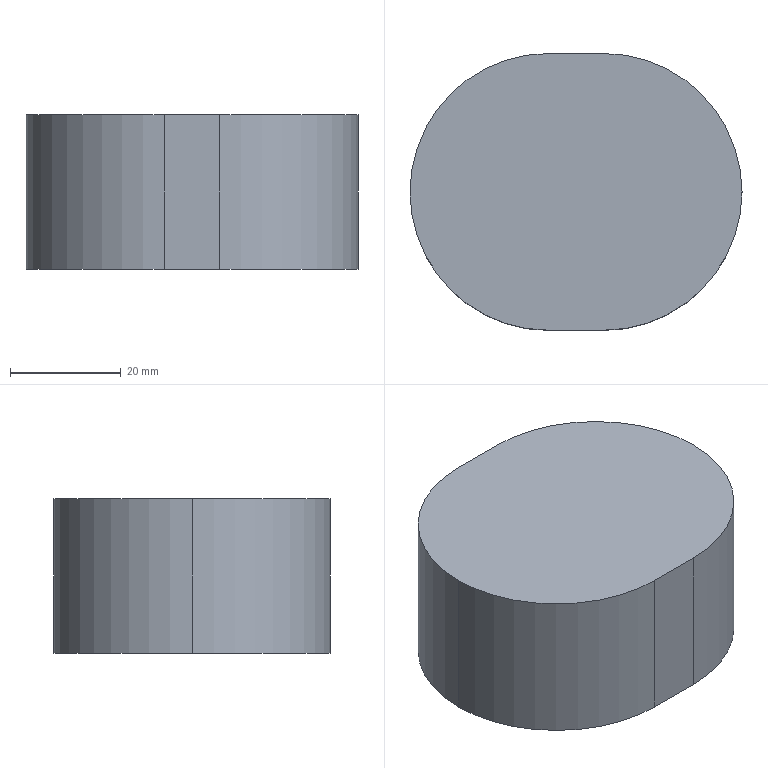Part | SolidWorks | features Extrusion 1, Fillet 1 | 1 solid | 8 faces | box 60 x 50 x 28 mm | volume 68978 mm3 | plane 4 | cylinder 4 | commonest cylinder face diameters 50 x4
STEP:
#1=CARTESIAN_POINT('',(5.,25.,28.));
#2=VERTEX_POINT('',#1);
#3=CARTESIAN_POINT('',(-5.,25.,28.));
#4=VERTEX_POINT('',#3);
#5=CARTESIAN_POINT('',(-30.,25.,28.));
#6=DIRECTION('',(-1.,0.,0.));
#7=VECTOR('',#6,1000.);
#8=LINE('',#5,#7);
#9=EDGE_CURVE('',#2,#4,#8,.T.);
#10=ORIENTED_EDGE('',*,*,#9,.F.);
#11=CARTESIAN_POINT('',(5.,25.,0.));
#12=VERTEX_POINT('',#11);
#13=CARTESIAN_POINT('',(5.,25.,28.));
#14=DIRECTION('',(0.,0.,-1.));
#15=VECTOR('',#14,1000.);
#16=LINE('',#13,#15);
#17=EDGE_CURVE('',#2,#12,#16,.T.);
#18=ORIENTED_EDGE('',*,*,#17,.T.);
#19=CARTESIAN_POINT('',(-5.,25.,0.));
#20=VERTEX_POINT('',#19);
#21=CARTESIAN_POINT('',(-30.,25.,0.));
#22=DIRECTION('',(-1.,0.,0.));
#23=VECTOR('',#22,1000.);
#24=LINE('',#21,#23);
#25=EDGE_CURVE('',#12,#20,#24,.T.);
#26=ORIENTED_EDGE('',*,*,#25,.T.);
#27=CARTESIAN_POINT('',(-5.,25.,28.));
#28=DIRECTION('',(0.,0.,1.));
#29=VECTOR('',#28,1000.);
#30=LINE('',#27,#29);
#31=EDGE_CURVE('',#20,#4,#30,.T.);
#32=ORIENTED_EDGE('',*,*,#31,.T.);
#33=EDGE_LOOP('',(#10,#18,#26,#32));
#34=FACE_OUTER_BOUND('',#33,.T.);
#35=CARTESIAN_POINT('',(-30.,25.,28.));
#36=DIRECTION('',(0.,-1.,0.));
#37=DIRECTION('',(0.,0.,-1.));
#38=AXIS2_PLACEMENT_3D('',#35,#36,#37);
#39=PLANE('',#38);
#40=ADVANCED_FACE('',(#34),#39,.F.);
#41=CARTESIAN_POINT('',(-5.,-25.,0.));
#42=VERTEX_POINT('',#41);
#43=CARTESIAN_POINT('',(5.,-25.,0.));
#44=VERTEX_POINT('',#43);
#45=CARTESIAN_POINT('',(-30.,-25.,0.));
#46=DIRECTION('',(1.,0.,0.));
#47=VECTOR('',#46,1000.);
#48=LINE('',#45,#47);
#49=EDGE_CURVE('',#42,#44,#48,.T.);
#50=ORIENTED_EDGE('',*,*,#49,.T.);
#51=CARTESIAN_POINT('',(5.,-25.,28.));
#52=VERTEX_POINT('',#51);
#53=CARTESIAN_POINT('',(5.,-25.,28.));
#54=DIRECTION('',(0.,0.,1.));
#55=VECTOR('',#54,1000.);
#56=LINE('',#53,#55);
#57=EDGE_CURVE('',#44,#52,#56,.T.);
#58=ORIENTED_EDGE('',*,*,#57,.T.);
#59=CARTESIAN_POINT('',(-5.,-25.,28.));
#60=VERTEX_POINT('',#59);
#61=CARTESIAN_POINT('',(-30.,-25.,28.));
#62=DIRECTION('',(1.,0.,0.));
#63=VECTOR('',#62,1000.);
#64=LINE('',#61,#63);
#65=EDGE_CURVE('',#60,#52,#64,.T.);
#66=ORIENTED_EDGE('',*,*,#65,.F.);
#67=CARTESIAN_POINT('',(-5.,-25.,28.));
#68=DIRECTION('',(0.,0.,-1.));
#69=VECTOR('',#68,1000.);
#70=LINE('',#67,#69);
#71=EDGE_CURVE('',#60,#42,#70,.T.);
#72=ORIENTED_EDGE('',*,*,#71,.T.);
#73=EDGE_LOOP('',(#50,#58,#66,#72));
#74=FACE_OUTER_BOUND('',#73,.T.);
#75=CARTESIAN_POINT('',(-30.,-25.,28.));
#76=DIRECTION('',(0.,1.,0.));
#77=DIRECTION('',(0.,0.,1.));
#78=AXIS2_PLACEMENT_3D('',#75,#76,#77);
#79=PLANE('',#78);
#80=ADVANCED_FACE('',(#74),#79,.F.);
#81=ORIENTED_EDGE('',*,*,#65,.T.);
#82=CARTESIAN_POINT('',(30.,0.,28.));
#83=VERTEX_POINT('',#82);
#84=CARTESIAN_POINT('',(5.,0.,28.));
#85=DIRECTION('',(0.,0.,1.));
#86=DIRECTION('',(1.,0.,0.));
#87=AXIS2_PLACEMENT_3D('',#84,#85,#86);
#88=CIRCLE('',#87,25.);
#89=EDGE_CURVE('',#52,#83,#88,.T.);
#90=ORIENTED_EDGE('',*,*,#89,.T.);
#91=CARTESIAN_POINT('',(5.,0.,28.));
#92=DIRECTION('',(0.,0.,1.));
#93=DIRECTION('',(1.,0.,0.));
#94=AXIS2_PLACEMENT_3D('',#91,#92,#93);
#95=CIRCLE('',#94,25.);
#96=EDGE_CURVE('',#83,#2,#95,.T.);
#97=ORIENTED_EDGE('',*,*,#96,.T.);
#98=ORIENTED_EDGE('',*,*,#9,.T.);
#99=CARTESIAN_POINT('',(-30.,0.,28.));
#100=VERTEX_POINT('',#99);
#101=CARTESIAN_POINT('',(-5.,0.,28.));
#102=DIRECTION('',(0.,0.,1.));
#103=DIRECTION('',(1.,0.,0.));
#104=AXIS2_PLACEMENT_3D('',#101,#102,#103);
#105=CIRCLE('',#104,25.);
#106=EDGE_CURVE('',#4,#100,#105,.T.);
#107=ORIENTED_EDGE('',*,*,#106,.T.);
#108=CARTESIAN_POINT('',(-5.,0.,28.));
#109=DIRECTION('',(0.,0.,1.));
#110=DIRECTION('',(1.,0.,0.));
#111=AXIS2_PLACEMENT_3D('',#108,#109,#110);
#112=CIRCLE('',#111,25.);
#113=EDGE_CURVE('',#100,#60,#112,.T.);
#114=ORIENTED_EDGE('',*,*,#113,.T.);
#115=EDGE_LOOP('',(#81,#90,#97,#98,#107,#114));
#116=FACE_OUTER_BOUND('',#115,.T.);
#117=CARTESIAN_POINT('',(0.,0.,28.));
#118=DIRECTION('',(0.,0.,1.));
#119=DIRECTION('',(1.,0.,0.));
#120=AXIS2_PLACEMENT_3D('',#117,#118,#119);
#121=PLANE('',#120);
#122=ADVANCED_FACE('',(#116),#121,.T.);
#123=CARTESIAN_POINT('',(30.,0.,0.));
#124=VERTEX_POINT('',#123);
#125=CARTESIAN_POINT('',(5.,0.,0.));
#126=DIRECTION('',(0.,0.,-1.));
#127=DIRECTION('',(1.,0.,0.));
#128=AXIS2_PLACEMENT_3D('',#125,#126,#127);
#129=CIRCLE('',#128,25.);
#130=EDGE_CURVE('',#12,#124,#129,.T.);
#131=ORIENTED_EDGE('',*,*,#130,.T.);
#132=CARTESIAN_POINT('',(5.,0.,0.));
#133=DIRECTION('',(0.,0.,-1.));
#134=DIRECTION('',(1.,0.,0.));
#135=AXIS2_PLACEMENT_3D('',#132,#133,#134);
#136=CIRCLE('',#135,25.);
#137=EDGE_CURVE('',#124,#44,#136,.T.);
#138=ORIENTED_EDGE('',*,*,#137,.T.);
#139=ORIENTED_EDGE('',*,*,#49,.F.);
#140=CARTESIAN_POINT('',(-30.,0.,0.));
#141=VERTEX_POINT('',#140);
#142=CARTESIAN_POINT('',(-5.,0.,0.));
#143=DIRECTION('',(0.,0.,-1.));
#144=DIRECTION('',(1.,0.,0.));
#145=AXIS2_PLACEMENT_3D('',#142,#143,#144);
#146=CIRCLE('',#145,25.);
#147=EDGE_CURVE('',#42,#141,#146,.T.);
#148=ORIENTED_EDGE('',*,*,#147,.T.);
#149=CARTESIAN_POINT('',(-5.,0.,0.));
#150=DIRECTION('',(0.,0.,-1.));
#151=DIRECTION('',(1.,0.,0.));
#152=AXIS2_PLACEMENT_3D('',#149,#150,#151);
#153=CIRCLE('',#152,25.);
#154=EDGE_CURVE('',#141,#20,#153,.T.);
#155=ORIENTED_EDGE('',*,*,#154,.T.);
#156=ORIENTED_EDGE('',*,*,#25,.F.);
#157=EDGE_LOOP('',(#131,#138,#139,#148,#155,#156));
#158=FACE_OUTER_BOUND('',#157,.T.);
#159=CARTESIAN_POINT('',(0.,0.,0.));
#160=DIRECTION('',(0.,0.,1.));
#161=DIRECTION('',(1.,0.,0.));
#162=AXIS2_PLACEMENT_3D('',#159,#160,#161);
#163=PLANE('',#162);
#164=ADVANCED_FACE('',(#158),#163,.F.);
#165=ORIENTED_EDGE('',*,*,#17,.F.);
#166=ORIENTED_EDGE('',*,*,#96,.F.);
#167=CARTESIAN_POINT('',(30.,0.,28.));
#168=DIRECTION('',(0.,0.,1.));
#169=VECTOR('',#168,1000.);
#170=LINE('',#167,#169);
#171=EDGE_CURVE('',#124,#83,#170,.T.);
#172=ORIENTED_EDGE('',*,*,#171,.F.);
#173=ORIENTED_EDGE('',*,*,#130,.F.);
#174=EDGE_LOOP('',(#165,#166,#172,#173));
#175=FACE_OUTER_BOUND('',#174,.T.);
#176=CARTESIAN_POINT('',(5.,0.,28.));
#177=DIRECTION('',(0.,0.,-1.));
#178=DIRECTION('',(-1.,0.,0.));
#179=AXIS2_PLACEMENT_3D('',#176,#177,#178);
#180=CYLINDRICAL_SURFACE('',#179,25.);
#181=ADVANCED_FACE('',(#175),#180,.T.);
#182=ORIENTED_EDGE('',*,*,#89,.F.);
#183=ORIENTED_EDGE('',*,*,#57,.F.);
#184=ORIENTED_EDGE('',*,*,#137,.F.);
#185=ORIENTED_EDGE('',*,*,#171,.T.);
#186=EDGE_LOOP('',(#182,#183,#184,#185));
#187=FACE_OUTER_BOUND('',#186,.T.);
#188=CARTESIAN_POINT('',(5.,0.,28.));
#189=DIRECTION('',(0.,0.,-1.));
#190=DIRECTION('',(-1.,0.,0.));
#191=AXIS2_PLACEMENT_3D('',#188,#189,#190);
#192=CYLINDRICAL_SURFACE('',#191,25.);
#193=ADVANCED_FACE('',(#187),#192,.T.);
#194=CARTESIAN_POINT('',(-30.,0.,28.));
#195=DIRECTION('',(0.,0.,-1.));
#196=VECTOR('',#195,1000.);
#197=LINE('',#194,#196);
#198=EDGE_CURVE('',#100,#141,#197,.T.);
#199=ORIENTED_EDGE('',*,*,#198,.F.);
#200=ORIENTED_EDGE('',*,*,#106,.F.);
#201=ORIENTED_EDGE('',*,*,#31,.F.);
#202=ORIENTED_EDGE('',*,*,#154,.F.);
#203=EDGE_LOOP('',(#199,#200,#201,#202));
#204=FACE_OUTER_BOUND('',#203,.T.);
#205=CARTESIAN_POINT('',(-5.,0.,28.));
#206=DIRECTION('',(0.,0.,-1.));
#207=DIRECTION('',(-1.,0.,0.));
#208=AXIS2_PLACEMENT_3D('',#205,#206,#207);
#209=CYLINDRICAL_SURFACE('',#208,25.);
#210=ADVANCED_FACE('',(#204),#209,.T.);
#211=ORIENTED_EDGE('',*,*,#113,.F.);
#212=ORIENTED_EDGE('',*,*,#198,.T.);
#213=ORIENTED_EDGE('',*,*,#147,.F.);
#214=ORIENTED_EDGE('',*,*,#71,.F.);
#215=EDGE_LOOP('',(#211,#212,#213,#214));
#216=FACE_OUTER_BOUND('',#215,.T.);
#217=CARTESIAN_POINT('',(-5.,0.,28.));
#218=DIRECTION('',(0.,0.,-1.));
#219=DIRECTION('',(-1.,0.,0.));
#220=AXIS2_PLACEMENT_3D('',#217,#218,#219);
#221=CYLINDRICAL_SURFACE('',#220,25.);
#222=ADVANCED_FACE('',(#216),#221,.T.);
#223=CLOSED_SHELL('',(#40,#80,#122,#164,#181,#193,#210,#222));
#224=MANIFOLD_SOLID_BREP('',#223);
#225=CARTESIAN_POINT('',(0.,0.,0.));
#226=DIRECTION('',(0.,0.,1.));
#227=DIRECTION('',(1.,0.,0.));
#228=AXIS2_PLACEMENT_3D('',#225,#226,#227);
#229=(LENGTH_UNIT()NAMED_UNIT(*)SI_UNIT(.MILLI.,.METRE.));
#230=UNCERTAINTY_MEASURE_WITH_UNIT(LENGTH_MEASURE(0.00001),#229,'','');
#231=(NAMED_UNIT(*)PLANE_ANGLE_UNIT()SI_UNIT($,.RADIAN.));
#232=(NAMED_UNIT(*)SI_UNIT($,.STERADIAN.)SOLID_ANGLE_UNIT());
#233=(GEOMETRIC_REPRESENTATION_CONTEXT(3)GLOBAL_UNCERTAINTY_ASSIGNED_CONTEXT((#230))GLOBAL_UNIT_ASSIGNED_CONTEXT((#229,#231,#232))REPRESENTATION_CONTEXT('',''));
#234=ADVANCED_BREP_SHAPE_REPRESENTATION('',(#224,#228),#233);